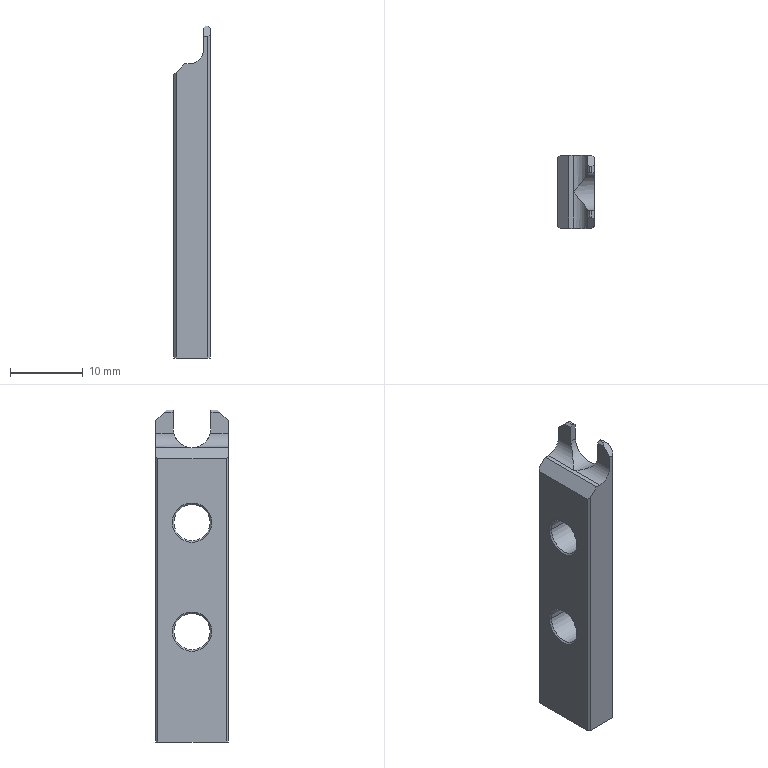Part | NX | 1 solid | 35 faces | box 5 x 10 x 45.7 mm | volume 1838 mm3 | plane 24 | cylinder 7 | cone 4 | commonest cylinder face diameters 5 x4 4 x2 5.2 x1
STEP:
#1=CARTESIAN_POINT('',(2162.7,155.748,-162.7));
#2=VERTEX_POINT('',#1);
#3=CARTESIAN_POINT('',(2163.,156.048,-162.7));
#4=VERTEX_POINT('',#3);
#5=CARTESIAN_POINT('',(2006.952,0.,-162.7));
#6=DIRECTION('',(0.7071,0.7071,0.));
#7=VECTOR('',#6,1000.);
#8=LINE('',#5,#7);
#9=EDGE_CURVE('',#2,#4,#8,.T.);
#10=ORIENTED_EDGE('',*,*,#9,.F.);
#11=CARTESIAN_POINT('',(2158.3,155.748,-162.7));
#12=VERTEX_POINT('',#11);
#13=CARTESIAN_POINT('',(0.,155.748,-162.7));
#14=DIRECTION('',(-1.,0.,0.));
#15=VECTOR('',#14,1000.);
#16=LINE('',#13,#15);
#17=EDGE_CURVE('',#2,#12,#16,.T.);
#18=ORIENTED_EDGE('',*,*,#17,.T.);
#19=CARTESIAN_POINT('',(2158.,156.048,-162.7));
#20=VERTEX_POINT('',#19);
#21=CARTESIAN_POINT('',(2314.048,0.,-162.7));
#22=DIRECTION('',(0.7071,-0.7071,0.));
#23=VECTOR('',#22,1000.);
#24=LINE('',#21,#23);
#25=EDGE_CURVE('',#20,#12,#24,.T.);
#26=ORIENTED_EDGE('',*,*,#25,.F.);
#27=CARTESIAN_POINT('',(2158.,165.448,-162.7));
#28=VERTEX_POINT('',#27);
#29=CARTESIAN_POINT('',(2158.,0.,-162.7));
#30=DIRECTION('',(0.,1.,0.));
#31=VECTOR('',#30,1000.);
#32=LINE('',#29,#31);
#33=EDGE_CURVE('',#20,#28,#32,.T.);
#34=ORIENTED_EDGE('',*,*,#33,.T.);
#35=CARTESIAN_POINT('',(2158.3,165.748,-162.7));
#36=VERTEX_POINT('',#35);
#37=CARTESIAN_POINT('',(1992.552,0.,-162.7));
#38=DIRECTION('',(-0.7071,-0.7071,0.));
#39=VECTOR('',#38,1000.);
#40=LINE('',#37,#39);
#41=EDGE_CURVE('',#36,#28,#40,.T.);
#42=ORIENTED_EDGE('',*,*,#41,.F.);
#43=CARTESIAN_POINT('',(2162.7,165.748,-162.7));
#44=VERTEX_POINT('',#43);
#45=CARTESIAN_POINT('',(0.,165.748,-162.7));
#46=DIRECTION('',(1.,0.,0.));
#47=VECTOR('',#46,1000.);
#48=LINE('',#45,#47);
#49=EDGE_CURVE('',#36,#44,#48,.T.);
#50=ORIENTED_EDGE('',*,*,#49,.T.);
#51=CARTESIAN_POINT('',(2163.,165.448,-162.7));
#52=VERTEX_POINT('',#51);
#53=CARTESIAN_POINT('',(2328.448,0.,-162.7));
#54=DIRECTION('',(0.7071,-0.7071,0.));
#55=VECTOR('',#54,1000.);
#56=LINE('',#53,#55);
#57=EDGE_CURVE('',#44,#52,#56,.T.);
#58=ORIENTED_EDGE('',*,*,#57,.T.);
#59=CARTESIAN_POINT('',(2163.,0.,-162.7));
#60=DIRECTION('',(0.,-1.,0.));
#61=VECTOR('',#60,1000.);
#62=LINE('',#59,#61);
#63=EDGE_CURVE('',#52,#4,#62,.T.);
#64=ORIENTED_EDGE('',*,*,#63,.T.);
#65=EDGE_LOOP('',(#10,#18,#26,#34,#42,#50,#58,#64));
#66=FACE_BOUND('',#65,.T.);
#67=CARTESIAN_POINT('',(2165.941,163.53,-162.7));
#68=DIRECTION('',(0.,0.,-1.));
#69=DIRECTION('',(0.,-1.,0.));
#70=AXIS2_PLACEMENT_3D('',#67,#68,#69);
#71=PLANE('',#70);
#72=ADVANCED_FACE('',(#66),#71,.T.);
#73=CARTESIAN_POINT('',(2162.7,155.748,-118.5));
#74=VERTEX_POINT('',#73);
#75=CARTESIAN_POINT('',(2162.7,155.748,0.));
#76=DIRECTION('',(0.,0.,1.));
#77=VECTOR('',#76,1000.);
#78=LINE('',#75,#77);
#79=EDGE_CURVE('',#2,#74,#78,.T.);
#80=ORIENTED_EDGE('',*,*,#79,.T.);
#81=CARTESIAN_POINT('',(2162.1,155.748,-118.5));
#82=VERTEX_POINT('',#81);
#83=CARTESIAN_POINT('',(2162.55,155.748,-118.5));
#84=DIRECTION('',(1.,0.,0.));
#85=VECTOR('',#84,1000.);
#86=LINE('',#83,#85);
#87=EDGE_CURVE('',#82,#74,#86,.T.);
#88=ORIENTED_EDGE('',*,*,#87,.F.);
#89=CARTESIAN_POINT('',(2162.1,155.748,-120.2));
#90=VERTEX_POINT('',#89);
#91=CARTESIAN_POINT('',(2162.1,155.748,-172.));
#92=DIRECTION('',(0.,0.,1.));
#93=VECTOR('',#92,1000.);
#94=LINE('',#91,#93);
#95=EDGE_CURVE('',#90,#82,#94,.T.);
#96=ORIENTED_EDGE('',*,*,#95,.F.);
#97=CARTESIAN_POINT('',(2160.1,155.748,-122.2));
#98=VERTEX_POINT('',#97);
#99=CARTESIAN_POINT('',(2160.1,155.748,-120.2));
#100=DIRECTION('',(0.,1.,0.));
#101=DIRECTION('',(-1.,0.,0.));
#102=AXIS2_PLACEMENT_3D('',#99,#100,#101);
#103=CIRCLE('',#102,2.);
#104=EDGE_CURVE('',#90,#98,#103,.T.);
#105=ORIENTED_EDGE('',*,*,#104,.T.);
#106=CARTESIAN_POINT('',(2159.5,155.748,-122.2));
#107=VERTEX_POINT('',#106);
#108=CARTESIAN_POINT('',(2165.941,155.748,-122.2));
#109=DIRECTION('',(1.,0.,0.));
#110=VECTOR('',#109,1000.);
#111=LINE('',#108,#110);
#112=EDGE_CURVE('',#107,#98,#111,.T.);
#113=ORIENTED_EDGE('',*,*,#112,.F.);
#114=CARTESIAN_POINT('',(2158.3,155.748,-123.4));
#115=VERTEX_POINT('',#114);
#116=CARTESIAN_POINT('',(2109.7,155.748,-172.));
#117=DIRECTION('',(-0.7071,0.,-0.7071));
#118=VECTOR('',#117,1000.);
#119=LINE('',#116,#118);
#120=EDGE_CURVE('',#107,#115,#119,.T.);
#121=ORIENTED_EDGE('',*,*,#120,.T.);
#122=CARTESIAN_POINT('',(2158.3,155.748,0.));
#123=DIRECTION('',(0.,0.,1.));
#124=VECTOR('',#123,1000.);
#125=LINE('',#122,#124);
#126=EDGE_CURVE('',#12,#115,#125,.T.);
#127=ORIENTED_EDGE('',*,*,#126,.F.);
#128=ORIENTED_EDGE('',*,*,#17,.F.);
#129=EDGE_LOOP('',(#80,#88,#96,#105,#113,#121,#127,#128));
#130=FACE_BOUND('',#129,.T.);
#131=CARTESIAN_POINT('',(2163.,155.748,-172.));
#132=DIRECTION('',(0.,-1.,0.));
#133=DIRECTION('',(0.,0.,-1.));
#134=AXIS2_PLACEMENT_3D('',#131,#132,#133);
#135=PLANE('',#134);
#136=ADVANCED_FACE('',(#130),#135,.T.);
#137=CARTESIAN_POINT('',(2163.,165.448,-118.2));
#138=VERTEX_POINT('',#137);
#139=CARTESIAN_POINT('',(2163.,165.448,0.));
#140=DIRECTION('',(0.,0.,1.));
#141=VECTOR('',#140,1000.);
#142=LINE('',#139,#141);
#143=EDGE_CURVE('',#52,#138,#142,.T.);
#144=ORIENTED_EDGE('',*,*,#143,.T.);
#145=CARTESIAN_POINT('',(2163.,164.548,-117.3));
#146=VERTEX_POINT('',#145);
#147=CARTESIAN_POINT('',(2163.,47.248,0.));
#148=DIRECTION('',(0.,-0.7071,0.7071));
#149=VECTOR('',#148,1000.);
#150=LINE('',#147,#149);
#151=EDGE_CURVE('',#138,#146,#150,.T.);
#152=ORIENTED_EDGE('',*,*,#151,.T.);
#153=CARTESIAN_POINT('',(2163.,163.348,-117.3));
#154=VERTEX_POINT('',#153);
#155=CARTESIAN_POINT('',(2163.,0.,-117.3));
#156=DIRECTION('',(0.,1.,0.));
#157=VECTOR('',#156,1000.);
#158=LINE('',#155,#157);
#159=EDGE_CURVE('',#154,#146,#158,.T.);
#160=ORIENTED_EDGE('',*,*,#159,.F.);
#161=CARTESIAN_POINT('',(2163.,163.348,-119.6));
#162=VERTEX_POINT('',#161);
#163=CARTESIAN_POINT('',(2163.,163.348,0.));
#164=DIRECTION('',(0.,0.,1.));
#165=VECTOR('',#164,1000.);
#166=LINE('',#163,#165);
#167=EDGE_CURVE('',#162,#154,#166,.T.);
#168=ORIENTED_EDGE('',*,*,#167,.F.);
#169=CARTESIAN_POINT('',(2163.,158.148,-119.6));
#170=VERTEX_POINT('',#169);
#171=CARTESIAN_POINT('',(2163.,160.748,-119.6));
#172=DIRECTION('',(1.,0.,0.));
#173=DIRECTION('',(0.,1.,0.));
#174=AXIS2_PLACEMENT_3D('',#171,#172,#173);
#175=CIRCLE('',#174,2.6);
#176=EDGE_CURVE('',#170,#162,#175,.T.);
#177=ORIENTED_EDGE('',*,*,#176,.F.);
#178=CARTESIAN_POINT('',(2163.,158.148,-117.3));
#179=VERTEX_POINT('',#178);
#180=CARTESIAN_POINT('',(2163.,158.148,0.));
#181=DIRECTION('',(0.,0.,-1.));
#182=VECTOR('',#181,1000.);
#183=LINE('',#180,#182);
#184=EDGE_CURVE('',#179,#170,#183,.T.);
#185=ORIENTED_EDGE('',*,*,#184,.F.);
#186=CARTESIAN_POINT('',(2163.,156.948,-117.3));
#187=VERTEX_POINT('',#186);
#188=CARTESIAN_POINT('',(2163.,156.948,-117.3));
#189=DIRECTION('',(0.,1.,0.));
#190=VECTOR('',#189,1000.);
#191=LINE('',#188,#190);
#192=EDGE_CURVE('',#187,#179,#191,.T.);
#193=ORIENTED_EDGE('',*,*,#192,.F.);
#194=CARTESIAN_POINT('',(2163.,156.048,-118.2));
#195=VERTEX_POINT('',#194);
#196=CARTESIAN_POINT('',(2163.,274.248,0.));
#197=DIRECTION('',(0.,-0.7071,-0.7071));
#198=VECTOR('',#197,1000.);
#199=LINE('',#196,#198);
#200=EDGE_CURVE('',#187,#195,#199,.T.);
#201=ORIENTED_EDGE('',*,*,#200,.T.);
#202=CARTESIAN_POINT('',(2163.,156.048,0.));
#203=DIRECTION('',(0.,0.,1.));
#204=VECTOR('',#203,1000.);
#205=LINE('',#202,#204);
#206=EDGE_CURVE('',#4,#195,#205,.T.);
#207=ORIENTED_EDGE('',*,*,#206,.F.);
#208=ORIENTED_EDGE('',*,*,#63,.F.);
#209=EDGE_LOOP('',(#144,#152,#160,#168,#177,#185,#193,#201,#207,#208));
#210=FACE_BOUND('',#209,.T.);
#211=CARTESIAN_POINT('',(2163.,158.248,-147.5));
#212=VERTEX_POINT('',#211);
#213=CARTESIAN_POINT('',(2163.,163.248,-147.5));
#214=VERTEX_POINT('',#213);
#215=CARTESIAN_POINT('',(2163.,160.748,-147.5));
#216=DIRECTION('',(-1.,0.,0.));
#217=DIRECTION('',(0.,-1.,0.));
#218=AXIS2_PLACEMENT_3D('',#215,#216,#217);
#219=CIRCLE('',#218,2.5);
#220=EDGE_CURVE('',#212,#214,#219,.T.);
#221=ORIENTED_EDGE('',*,*,#220,.T.);
#222=CARTESIAN_POINT('',(2163.,160.748,-147.5));
#223=DIRECTION('',(-1.,0.,0.));
#224=DIRECTION('',(0.,-1.,0.));
#225=AXIS2_PLACEMENT_3D('',#222,#223,#224);
#226=CIRCLE('',#225,2.5);
#227=EDGE_CURVE('',#214,#212,#226,.T.);
#228=ORIENTED_EDGE('',*,*,#227,.T.);
#229=EDGE_LOOP('',(#221,#228));
#230=FACE_BOUND('',#229,.T.);
#231=CARTESIAN_POINT('',(2163.,158.248,-132.5));
#232=VERTEX_POINT('',#231);
#233=CARTESIAN_POINT('',(2163.,163.248,-132.5));
#234=VERTEX_POINT('',#233);
#235=CARTESIAN_POINT('',(2163.,160.748,-132.5));
#236=DIRECTION('',(-1.,0.,0.));
#237=DIRECTION('',(0.,-1.,0.));
#238=AXIS2_PLACEMENT_3D('',#235,#236,#237);
#239=CIRCLE('',#238,2.5);
#240=EDGE_CURVE('',#232,#234,#239,.T.);
#241=ORIENTED_EDGE('',*,*,#240,.T.);
#242=CARTESIAN_POINT('',(2163.,160.748,-132.5));
#243=DIRECTION('',(-1.,0.,0.));
#244=DIRECTION('',(0.,-1.,0.));
#245=AXIS2_PLACEMENT_3D('',#242,#243,#244);
#246=CIRCLE('',#245,2.5);
#247=EDGE_CURVE('',#234,#232,#246,.T.);
#248=ORIENTED_EDGE('',*,*,#247,.T.);
#249=EDGE_LOOP('',(#241,#248));
#250=FACE_BOUND('',#249,.T.);
#251=CARTESIAN_POINT('',(2163.,165.748,-172.));
#252=DIRECTION('',(1.,0.,0.));
#253=DIRECTION('',(0.,1.,0.));
#254=AXIS2_PLACEMENT_3D('',#251,#252,#253);
#255=PLANE('',#254);
#256=ADVANCED_FACE('',(#210,#230,#250),#255,.T.);
#257=CARTESIAN_POINT('',(2158.3,165.748,-123.4));
#258=VERTEX_POINT('',#257);
#259=CARTESIAN_POINT('',(2158.3,165.748,-155.));
#260=DIRECTION('',(0.,0.,-1.));
#261=VECTOR('',#260,1000.);
#262=LINE('',#259,#261);
#263=EDGE_CURVE('',#258,#36,#262,.T.);
#264=ORIENTED_EDGE('',*,*,#263,.F.);
#265=CARTESIAN_POINT('',(2159.5,165.748,-122.2));
#266=VERTEX_POINT('',#265);
#267=CARTESIAN_POINT('',(2109.7,165.748,-172.));
#268=DIRECTION('',(0.7071,0.,0.7071));
#269=VECTOR('',#268,1000.);
#270=LINE('',#267,#269);
#271=EDGE_CURVE('',#258,#266,#270,.T.);
#272=ORIENTED_EDGE('',*,*,#271,.T.);
#273=CARTESIAN_POINT('',(2160.1,165.748,-122.2));
#274=VERTEX_POINT('',#273);
#275=CARTESIAN_POINT('',(2165.941,165.748,-122.2));
#276=DIRECTION('',(-1.,0.,0.));
#277=VECTOR('',#276,1000.);
#278=LINE('',#275,#277);
#279=EDGE_CURVE('',#274,#266,#278,.T.);
#280=ORIENTED_EDGE('',*,*,#279,.F.);
#281=CARTESIAN_POINT('',(2162.1,165.748,-120.2));
#282=VERTEX_POINT('',#281);
#283=CARTESIAN_POINT('',(2160.1,165.748,-120.2));
#284=DIRECTION('',(0.,1.,0.));
#285=DIRECTION('',(-1.,0.,0.));
#286=AXIS2_PLACEMENT_3D('',#283,#284,#285);
#287=CIRCLE('',#286,2.);
#288=EDGE_CURVE('',#282,#274,#287,.T.);
#289=ORIENTED_EDGE('',*,*,#288,.F.);
#290=CARTESIAN_POINT('',(2162.1,165.748,-118.5));
#291=VERTEX_POINT('',#290);
#292=CARTESIAN_POINT('',(2162.1,165.748,0.));
#293=DIRECTION('',(0.,0.,-1.));
#294=VECTOR('',#293,1000.);
#295=LINE('',#292,#294);
#296=EDGE_CURVE('',#291,#282,#295,.T.);
#297=ORIENTED_EDGE('',*,*,#296,.F.);
#298=CARTESIAN_POINT('',(2162.7,165.748,-118.5));
#299=VERTEX_POINT('',#298);
#300=CARTESIAN_POINT('',(2162.55,165.748,-118.5));
#301=DIRECTION('',(-1.,0.,0.));
#302=VECTOR('',#301,1000.);
#303=LINE('',#300,#302);
#304=EDGE_CURVE('',#299,#291,#303,.T.);
#305=ORIENTED_EDGE('',*,*,#304,.F.);
#306=CARTESIAN_POINT('',(2162.7,165.748,-155.));
#307=DIRECTION('',(0.,0.,-1.));
#308=VECTOR('',#307,1000.);
#309=LINE('',#306,#308);
#310=EDGE_CURVE('',#299,#44,#309,.T.);
#311=ORIENTED_EDGE('',*,*,#310,.T.);
#312=ORIENTED_EDGE('',*,*,#49,.F.);
#313=EDGE_LOOP('',(#264,#272,#280,#289,#297,#305,#311,#312));
#314=FACE_BOUND('',#313,.T.);
#315=CARTESIAN_POINT('',(2158.,165.748,-172.));
#316=DIRECTION('',(0.,1.,0.));
#317=DIRECTION('',(1.,0.,0.));
#318=AXIS2_PLACEMENT_3D('',#315,#316,#317);
#319=PLANE('',#318);
#320=ADVANCED_FACE('',(#314),#319,.T.);
#321=CARTESIAN_POINT('',(2158.,156.048,-123.7));
#322=VERTEX_POINT('',#321);
#323=CARTESIAN_POINT('',(2158.,156.048,-155.));
#324=DIRECTION('',(0.,0.,-1.));
#325=VECTOR('',#324,1000.);
#326=LINE('',#323,#325);
#327=EDGE_CURVE('',#322,#20,#326,.T.);
#328=ORIENTED_EDGE('',*,*,#327,.F.);
#329=CARTESIAN_POINT('',(2158.,165.448,-123.7));
#330=VERTEX_POINT('',#329);
#331=CARTESIAN_POINT('',(2158.,160.748,-123.7));
#332=DIRECTION('',(0.,-1.,0.));
#333=VECTOR('',#332,1000.);
#334=LINE('',#331,#333);
#335=EDGE_CURVE('',#330,#322,#334,.T.);
#336=ORIENTED_EDGE('',*,*,#335,.F.);
#337=CARTESIAN_POINT('',(2158.,165.448,0.));
#338=DIRECTION('',(0.,0.,1.));
#339=VECTOR('',#338,1000.);
#340=LINE('',#337,#339);
#341=EDGE_CURVE('',#28,#330,#340,.T.);
#342=ORIENTED_EDGE('',*,*,#341,.F.);
#343=ORIENTED_EDGE('',*,*,#33,.F.);
#344=EDGE_LOOP('',(#328,#336,#342,#343));
#345=FACE_BOUND('',#344,.T.);
#346=CARTESIAN_POINT('',(2158.,158.048,-147.5));
#347=VERTEX_POINT('',#346);
#348=CARTESIAN_POINT('',(2158.,163.448,-147.5));
#349=VERTEX_POINT('',#348);
#350=CARTESIAN_POINT('',(2158.,160.748,-147.5));
#351=DIRECTION('',(-1.,0.,0.));
#352=DIRECTION('',(0.,-1.,0.));
#353=AXIS2_PLACEMENT_3D('',#350,#351,#352);
#354=CIRCLE('',#353,2.7);
#355=EDGE_CURVE('',#347,#349,#354,.T.);
#356=ORIENTED_EDGE('',*,*,#355,.F.);
#357=CARTESIAN_POINT('',(2158.,160.748,-147.5));
#358=DIRECTION('',(-1.,0.,0.));
#359=DIRECTION('',(0.,-1.,0.));
#360=AXIS2_PLACEMENT_3D('',#357,#358,#359);
#361=CIRCLE('',#360,2.7);
#362=EDGE_CURVE('',#349,#347,#361,.T.);
#363=ORIENTED_EDGE('',*,*,#362,.F.);
#364=EDGE_LOOP('',(#356,#363));
#365=FACE_BOUND('',#364,.T.);
#366=CARTESIAN_POINT('',(2158.,163.448,-132.5));
#367=VERTEX_POINT('',#366);
#368=CARTESIAN_POINT('',(2158.,158.048,-132.5));
#369=VERTEX_POINT('',#368);
#370=CARTESIAN_POINT('',(2158.,160.748,-132.5));
#371=DIRECTION('',(-1.,0.,0.));
#372=DIRECTION('',(0.,-1.,0.));
#373=AXIS2_PLACEMENT_3D('',#370,#371,#372);
#374=CIRCLE('',#373,2.7);
#375=EDGE_CURVE('',#367,#369,#374,.T.);
#376=ORIENTED_EDGE('',*,*,#375,.F.);
#377=CARTESIAN_POINT('',(2158.,160.748,-132.5));
#378=DIRECTION('',(-1.,0.,0.));
#379=DIRECTION('',(0.,-1.,0.));
#380=AXIS2_PLACEMENT_3D('',#377,#378,#379);
#381=CIRCLE('',#380,2.7);
#382=EDGE_CURVE('',#369,#367,#381,.T.);
#383=ORIENTED_EDGE('',*,*,#382,.F.);
#384=EDGE_LOOP('',(#376,#383));
#385=FACE_BOUND('',#384,.T.);
#386=CARTESIAN_POINT('',(2158.,155.748,-172.));
#387=DIRECTION('',(-1.,0.,0.));
#388=DIRECTION('',(0.,0.,1.));
#389=AXIS2_PLACEMENT_3D('',#386,#387,#388);
#390=PLANE('',#389);
#391=ADVANCED_FACE('',(#345,#365,#385),#390,.T.);
#392=ORIENTED_EDGE('',*,*,#167,.T.);
#393=CARTESIAN_POINT('',(2162.7,163.348,-117.));
#394=VERTEX_POINT('',#393);
#395=CARTESIAN_POINT('',(0.,163.348,2045.7));
#396=DIRECTION('',(-0.7071,0.,0.7071));
#397=VECTOR('',#396,1000.);
#398=LINE('',#395,#397);
#399=EDGE_CURVE('',#154,#394,#398,.T.);
#400=ORIENTED_EDGE('',*,*,#399,.T.);
#401=CARTESIAN_POINT('',(2162.4,163.348,-117.));
#402=VERTEX_POINT('',#401);
#403=CARTESIAN_POINT('',(2162.1,163.348,-117.));
#404=DIRECTION('',(1.,0.,0.));
#405=VECTOR('',#404,1000.);
#406=LINE('',#403,#405);
#407=EDGE_CURVE('',#402,#394,#406,.T.);
#408=ORIENTED_EDGE('',*,*,#407,.F.);
#409=CARTESIAN_POINT('',(2162.1,163.348,-117.3));
#410=VERTEX_POINT('',#409);
#411=CARTESIAN_POINT('',(0.,163.348,-2279.4));
#412=DIRECTION('',(0.7071,0.,0.7071));
#413=VECTOR('',#412,1000.);
#414=LINE('',#411,#413);
#415=EDGE_CURVE('',#410,#402,#414,.T.);
#416=ORIENTED_EDGE('',*,*,#415,.F.);
#417=CARTESIAN_POINT('',(2162.1,163.348,-119.6));
#418=VERTEX_POINT('',#417);
#419=CARTESIAN_POINT('',(2162.1,163.348,0.));
#420=DIRECTION('',(0.,0.,1.));
#421=VECTOR('',#420,1000.);
#422=LINE('',#419,#421);
#423=EDGE_CURVE('',#418,#410,#422,.T.);
#424=ORIENTED_EDGE('',*,*,#423,.F.);
#425=CARTESIAN_POINT('',(2157.5,163.348,-119.6));
#426=DIRECTION('',(1.,0.,0.));
#427=VECTOR('',#426,1000.);
#428=LINE('',#425,#427);
#429=EDGE_CURVE('',#418,#162,#428,.T.);
#430=ORIENTED_EDGE('',*,*,#429,.T.);
#431=EDGE_LOOP('',(#392,#400,#408,#416,#424,#430));
#432=FACE_BOUND('',#431,.T.);
#433=CARTESIAN_POINT('',(2157.5,163.348,-117.));
#434=DIRECTION('',(0.,1.,0.));
#435=DIRECTION('',(0.,0.,-1.));
#436=AXIS2_PLACEMENT_3D('',#433,#434,#435);
#437=PLANE('',#436);
#438=ADVANCED_FACE('',(#432),#437,.F.);
#439=ORIENTED_EDGE('',*,*,#296,.T.);
#440=CARTESIAN_POINT('',(2162.1,163.277,-120.2));
#441=VERTEX_POINT('',#440);
#442=CARTESIAN_POINT('',(2162.1,163.53,-120.2));
#443=DIRECTION('',(0.,1.,0.));
#444=VECTOR('',#443,1000.);
#445=LINE('',#442,#444);
#446=EDGE_CURVE('',#441,#282,#445,.T.);
#447=ORIENTED_EDGE('',*,*,#446,.F.);
#448=CARTESIAN_POINT('',(2162.1,160.748,-119.6));
#449=DIRECTION('',(1.,0.,0.));
#450=DIRECTION('',(0.,1.,0.));
#451=AXIS2_PLACEMENT_3D('',#448,#449,#450);
#452=CIRCLE('',#451,2.6);
#453=EDGE_CURVE('',#441,#418,#452,.T.);
#454=ORIENTED_EDGE('',*,*,#453,.T.);
#455=ORIENTED_EDGE('',*,*,#423,.T.);
#456=CARTESIAN_POINT('',(2162.1,164.548,-117.3));
#457=VERTEX_POINT('',#456);
#458=CARTESIAN_POINT('',(2162.1,0.,-117.3));
#459=DIRECTION('',(0.,1.,0.));
#460=VECTOR('',#459,1000.);
#461=LINE('',#458,#460);
#462=EDGE_CURVE('',#410,#457,#461,.T.);
#463=ORIENTED_EDGE('',*,*,#462,.T.);
#464=CARTESIAN_POINT('',(2162.1,47.248,0.));
#465=DIRECTION('',(0.,-0.7071,0.7071));
#466=VECTOR('',#465,1000.);
#467=LINE('',#464,#466);
#468=EDGE_CURVE('',#291,#457,#467,.T.);
#469=ORIENTED_EDGE('',*,*,#468,.F.);
#470=EDGE_LOOP('',(#439,#447,#454,#455,#463,#469));
#471=FACE_BOUND('',#470,.T.);
#472=CARTESIAN_POINT('',(2162.1,154.748,-124.2));
#473=DIRECTION('',(1.,0.,0.));
#474=DIRECTION('',(0.,1.,0.));
#475=AXIS2_PLACEMENT_3D('',#472,#473,#474);
#476=PLANE('',#475);
#477=ADVANCED_FACE('',(#471),#476,.F.);
#478=CARTESIAN_POINT('',(2162.1,158.148,-117.3));
#479=VERTEX_POINT('',#478);
#480=CARTESIAN_POINT('',(2162.1,158.148,-119.6));
#481=VERTEX_POINT('',#480);
#482=CARTESIAN_POINT('',(2162.1,158.148,0.));
#483=DIRECTION('',(0.,0.,-1.));
#484=VECTOR('',#483,1000.);
#485=LINE('',#482,#484);
#486=EDGE_CURVE('',#479,#481,#485,.T.);
#487=ORIENTED_EDGE('',*,*,#486,.T.);
#488=CARTESIAN_POINT('',(2162.1,158.218,-120.2));
#489=VERTEX_POINT('',#488);
#490=CARTESIAN_POINT('',(2162.1,160.748,-119.6));
#491=DIRECTION('',(1.,0.,0.));
#492=DIRECTION('',(0.,1.,0.));
#493=AXIS2_PLACEMENT_3D('',#490,#491,#492);
#494=CIRCLE('',#493,2.6);
#495=EDGE_CURVE('',#481,#489,#494,.T.);
#496=ORIENTED_EDGE('',*,*,#495,.T.);
#497=CARTESIAN_POINT('',(2162.1,163.53,-120.2));
#498=DIRECTION('',(0.,1.,0.));
#499=VECTOR('',#498,1000.);
#500=LINE('',#497,#499);
#501=EDGE_CURVE('',#90,#489,#500,.T.);
#502=ORIENTED_EDGE('',*,*,#501,.F.);
#503=ORIENTED_EDGE('',*,*,#95,.T.);
#504=CARTESIAN_POINT('',(2162.1,156.948,-117.3));
#505=VERTEX_POINT('',#504);
#506=CARTESIAN_POINT('',(2162.1,274.248,0.));
#507=DIRECTION('',(0.,-0.7071,-0.7071));
#508=VECTOR('',#507,1000.);
#509=LINE('',#506,#508);
#510=EDGE_CURVE('',#505,#82,#509,.T.);
#511=ORIENTED_EDGE('',*,*,#510,.F.);
#512=CARTESIAN_POINT('',(2162.1,156.948,-117.3));
#513=DIRECTION('',(0.,1.,0.));
#514=VECTOR('',#513,1000.);
#515=LINE('',#512,#514);
#516=EDGE_CURVE('',#505,#479,#515,.T.);
#517=ORIENTED_EDGE('',*,*,#516,.T.);
#518=EDGE_LOOP('',(#487,#496,#502,#503,#511,#517));
#519=FACE_BOUND('',#518,.T.);
#520=CARTESIAN_POINT('',(2162.1,154.748,-124.2));
#521=DIRECTION('',(1.,0.,0.));
#522=DIRECTION('',(0.,1.,0.));
#523=AXIS2_PLACEMENT_3D('',#520,#521,#522);
#524=PLANE('',#523);
#525=ADVANCED_FACE('',(#519),#524,.F.);
#526=CARTESIAN_POINT('',(2159.5,160.748,-122.2));
#527=DIRECTION('',(0.,-1.,0.));
#528=VECTOR('',#527,1000.);
#529=LINE('',#526,#528);
#530=EDGE_CURVE('',#266,#107,#529,.T.);
#531=ORIENTED_EDGE('',*,*,#530,.T.);
#532=ORIENTED_EDGE('',*,*,#112,.T.);
#533=CARTESIAN_POINT('',(2160.1,160.748,-122.2));
#534=VERTEX_POINT('',#533);
#535=CARTESIAN_POINT('',(2160.1,163.53,-122.2));
#536=DIRECTION('',(0.,1.,0.));
#537=VECTOR('',#536,1000.);
#538=LINE('',#535,#537);
#539=EDGE_CURVE('',#98,#534,#538,.T.);
#540=ORIENTED_EDGE('',*,*,#539,.T.);
#541=CARTESIAN_POINT('',(2160.1,163.53,-122.2));
#542=DIRECTION('',(0.,1.,0.));
#543=VECTOR('',#542,1000.);
#544=LINE('',#541,#543);
#545=EDGE_CURVE('',#534,#274,#544,.T.);
#546=ORIENTED_EDGE('',*,*,#545,.T.);
#547=ORIENTED_EDGE('',*,*,#279,.T.);
#548=EDGE_LOOP('',(#531,#532,#540,#546,#547));
#549=FACE_BOUND('',#548,.T.);
#550=CARTESIAN_POINT('',(2158.,154.748,-122.2));
#551=DIRECTION('',(0.,0.,-1.));
#552=DIRECTION('',(0.,-1.,0.));
#553=AXIS2_PLACEMENT_3D('',#550,#551,#552);
#554=PLANE('',#553);
#555=ADVANCED_FACE('',(#549),#554,.F.);
#556=ORIENTED_EDGE('',*,*,#446,.T.);
#557=ORIENTED_EDGE('',*,*,#288,.T.);
#558=ORIENTED_EDGE('',*,*,#545,.F.);
#559=CARTESIAN_POINT('',(2160.1,160.748,-122.2));
#560=CARTESIAN_POINT('',(2160.212,160.876,-122.2));
#561=CARTESIAN_POINT('',(2160.325,161.004,-122.191));
#562=CARTESIAN_POINT('',(2160.436,161.131,-122.172));
#563=CARTESIAN_POINT('',(2160.492,161.195,-122.162));
#564=CARTESIAN_POINT('',(2160.547,161.259,-122.15));
#565=CARTESIAN_POINT('',(2160.603,161.322,-122.136));
#566=CARTESIAN_POINT('',(2160.63,161.354,-122.129));
#567=CARTESIAN_POINT('',(2160.658,161.385,-122.121));
#568=CARTESIAN_POINT('',(2160.685,161.417,-122.112));
#569=CARTESIAN_POINT('',(2160.713,161.448,-122.104));
#570=CARTESIAN_POINT('',(2160.74,161.48,-122.095));
#571=CARTESIAN_POINT('',(2160.767,161.511,-122.085));
#572=CARTESIAN_POINT('',(2160.822,161.574,-122.066));
#573=CARTESIAN_POINT('',(2160.876,161.636,-122.044));
#574=CARTESIAN_POINT('',(2160.929,161.698,-122.02));
#575=CARTESIAN_POINT('',(2160.982,161.76,-121.996));
#576=CARTESIAN_POINT('',(2161.035,161.821,-121.969));
#577=CARTESIAN_POINT('',(2161.087,161.882,-121.939));
#578=CARTESIAN_POINT('',(2161.113,161.913,-121.925));
#579=CARTESIAN_POINT('',(2161.139,161.943,-121.909));
#580=CARTESIAN_POINT('',(2161.164,161.973,-121.893));
#581=CARTESIAN_POINT('',(2161.19,162.003,-121.877));
#582=CARTESIAN_POINT('',(2161.215,162.033,-121.86));
#583=CARTESIAN_POINT('',(2161.24,162.063,-121.843));
#584=CARTESIAN_POINT('',(2161.291,162.122,-121.808));
#585=CARTESIAN_POINT('',(2161.34,162.181,-121.771));
#586=CARTESIAN_POINT('',(2161.388,162.239,-121.73));
#587=CARTESIAN_POINT('',(2161.436,162.296,-121.69));
#588=CARTESIAN_POINT('',(2161.483,162.353,-121.646));
#589=CARTESIAN_POINT('',(2161.528,162.409,-121.6));
#590=CARTESIAN_POINT('',(2161.551,162.436,-121.577));
#591=CARTESIAN_POINT('',(2161.573,162.464,-121.553));
#592=CARTESIAN_POINT('',(2161.595,162.491,-121.529));
#593=CARTESIAN_POINT('',(2161.617,162.519,-121.504));
#594=CARTESIAN_POINT('',(2161.638,162.546,-121.479));
#595=CARTESIAN_POINT('',(2161.659,162.572,-121.452));
#596=CARTESIAN_POINT('',(2161.68,162.599,-121.426));
#597=CARTESIAN_POINT('',(2161.701,162.625,-121.399));
#598=CARTESIAN_POINT('',(2161.721,162.651,-121.371));
#599=CARTESIAN_POINT('',(2161.741,162.677,-121.344));
#600=CARTESIAN_POINT('',(2161.761,162.702,-121.315));
#601=CARTESIAN_POINT('',(2161.78,162.727,-121.286));
#602=CARTESIAN_POINT('',(2161.799,162.752,-121.256));
#603=CARTESIAN_POINT('',(2161.817,162.777,-121.226));
#604=CARTESIAN_POINT('',(2161.835,162.801,-121.196));
#605=CARTESIAN_POINT('',(2161.852,162.824,-121.165));
#606=CARTESIAN_POINT('',(2161.869,162.848,-121.133));
#607=CARTESIAN_POINT('',(2161.886,162.871,-121.101));
#608=CARTESIAN_POINT('',(2161.902,162.893,-121.069));
#609=CARTESIAN_POINT('',(2161.917,162.916,-121.036));
#610=CARTESIAN_POINT('',(2161.932,162.937,-121.002));
#611=CARTESIAN_POINT('',(2161.947,162.959,-120.968));
#612=CARTESIAN_POINT('',(2161.961,162.98,-120.934));
#613=CARTESIAN_POINT('',(2161.974,163.,-120.899));
#614=CARTESIAN_POINT('',(2161.987,163.02,-120.864));
#615=CARTESIAN_POINT('',(2161.999,163.04,-120.828));
#616=CARTESIAN_POINT('',(2162.011,163.059,-120.791));
#617=CARTESIAN_POINT('',(2162.022,163.078,-120.754));
#618=CARTESIAN_POINT('',(2162.032,163.096,-120.717));
#619=CARTESIAN_POINT('',(2162.042,163.113,-120.679));
#620=CARTESIAN_POINT('',(2162.051,163.13,-120.641));
#621=CARTESIAN_POINT('',(2162.059,163.147,-120.603));
#622=CARTESIAN_POINT('',(2162.067,163.162,-120.564));
#623=CARTESIAN_POINT('',(2162.074,163.178,-120.525));
#624=CARTESIAN_POINT('',(2162.08,163.193,-120.485));
#625=CARTESIAN_POINT('',(2162.085,163.206,-120.445));
#626=CARTESIAN_POINT('',(2162.09,163.22,-120.405));
#627=CARTESIAN_POINT('',(2162.094,163.233,-120.364));
#628=CARTESIAN_POINT('',(2162.096,163.245,-120.324));
#629=CARTESIAN_POINT('',(2162.099,163.257,-120.283));
#630=CARTESIAN_POINT('',(2162.1,163.268,-120.241));
#631=CARTESIAN_POINT('',(2162.1,163.277,-120.2));
#632=B_SPLINE_CURVE_WITH_KNOTS('',3,(#559,#560,#561,#562,#563,#564,#565,#566,#567,#568,#569,#570,#571,#572,#573,#574,#575,#576,#577,#578,#579,#580,#581,#582,#583,#584,#585,#586,#587,#588,#589,#590,#591,#592,#593,#594,#595,#596,#597,#598,#599,#600,#601,#602,#603,#604,#605,#606,#607,#608,#609,#610,#611,#612,#613,#614,#615,#616,#617,#618,#619,#620,#621,#622,#623,#624,#625,#626,#627,#628,#629,#630,#631),.UNSPECIFIED.,.F.,.F.,(4,3,3,3,3,3,3,3,3,3,3,3,3,3,3,3,3,3,3,3,3,3,3,3,4),(0.,0.5111,0.7667,0.8945,1.022,1.278,1.534,1.662,1.79,2.046,2.301,2.43,2.558,2.687,2.816,2.944,3.073,3.201,3.329,3.457,3.585,3.713,3.841,3.969,4.097),.UNSPECIFIED.);
#633=EDGE_CURVE('',#534,#441,#632,.T.);
#634=ORIENTED_EDGE('',*,*,#633,.T.);
#635=EDGE_LOOP('',(#556,#557,#558,#634));
#636=FACE_BOUND('',#635,.T.);
#637=CARTESIAN_POINT('',(2160.1,163.53,-120.2));
#638=DIRECTION('',(0.,1.,0.));
#639=DIRECTION('',(-1.,0.,0.));
#640=AXIS2_PLACEMENT_3D('',#637,#638,#639);
#641=CYLINDRICAL_SURFACE('',#640,2.);
#642=ADVANCED_FACE('',(#636),#641,.F.);
#643=ORIENTED_EDGE('',*,*,#335,.T.);
#644=CARTESIAN_POINT('',(2109.7,204.348,-172.));
#645=DIRECTION('',(-0.5774,0.5774,-0.5774));
#646=VECTOR('',#645,1000.);
#647=LINE('',#644,#646);
#648=EDGE_CURVE('',#115,#322,#647,.T.);
#649=ORIENTED_EDGE('',*,*,#648,.F.);
#650=ORIENTED_EDGE('',*,*,#120,.F.);
#651=ORIENTED_EDGE('',*,*,#530,.F.);
#652=ORIENTED_EDGE('',*,*,#271,.F.);
#653=CARTESIAN_POINT('',(2156.083,163.53,-125.617));
#654=DIRECTION('',(-0.5774,-0.5774,-0.5774));
#655=VECTOR('',#654,1000.);
#656=LINE('',#653,#655);
#657=EDGE_CURVE('',#258,#330,#656,.T.);
#658=ORIENTED_EDGE('',*,*,#657,.T.);
#659=EDGE_LOOP('',(#643,#649,#650,#651,#652,#658));
#660=FACE_BOUND('',#659,.T.);
#661=CARTESIAN_POINT('',(2158.75,160.748,-122.95));
#662=DIRECTION('',(0.7071,0.,-0.7071));
#663=DIRECTION('',(0.,-1.,0.));
#664=AXIS2_PLACEMENT_3D('',#661,#662,#663);
#665=PLANE('',#664);
#666=ADVANCED_FACE('',(#660),#665,.F.);
#667=CARTESIAN_POINT('',(2158.2,163.248,-132.5));
#668=VERTEX_POINT('',#667);
#669=CARTESIAN_POINT('',(2158.2,158.248,-132.5));
#670=VERTEX_POINT('',#669);
#671=CARTESIAN_POINT('',(2158.2,160.748,-132.5));
#672=DIRECTION('',(-1.,0.,0.));
#673=DIRECTION('',(0.,-1.,0.));
#674=AXIS2_PLACEMENT_3D('',#671,#672,#673);
#675=CIRCLE('',#674,2.5);
#676=EDGE_CURVE('',#668,#670,#675,.T.);
#677=ORIENTED_EDGE('',*,*,#676,.T.);
#678=CARTESIAN_POINT('',(2158.,158.248,-132.5));
#679=DIRECTION('',(-1.,0.,0.));
#680=VECTOR('',#679,1000.);
#681=LINE('',#678,#680);
#682=EDGE_CURVE('',#670,#232,#681,.F.);
#683=ORIENTED_EDGE('',*,*,#682,.T.);
#684=ORIENTED_EDGE('',*,*,#247,.F.);
#685=CARTESIAN_POINT('',(2158.,163.248,-132.5));
#686=DIRECTION('',(-1.,0.,0.));
#687=VECTOR('',#686,1000.);
#688=LINE('',#685,#687);
#689=EDGE_CURVE('',#668,#234,#688,.F.);
#690=ORIENTED_EDGE('',*,*,#689,.F.);
#691=EDGE_LOOP('',(#677,#683,#684,#690));
#692=FACE_BOUND('',#691,.T.);
#693=CARTESIAN_POINT('',(2158.,160.748,-132.5));
#694=DIRECTION('',(-1.,0.,0.));
#695=DIRECTION('',(0.,-1.,0.));
#696=AXIS2_PLACEMENT_3D('',#693,#694,#695);
#697=CYLINDRICAL_SURFACE('',#696,2.5);
#698=ADVANCED_FACE('',(#692),#697,.F.);
#699=ORIENTED_EDGE('',*,*,#676,.F.);
#700=CARTESIAN_POINT('',(2158.2,163.248,-132.5));
#701=DIRECTION('',(-0.7071,0.7071,0.));
#702=VECTOR('',#701,1000.);
#703=LINE('',#700,#702);
#704=EDGE_CURVE('',#668,#367,#703,.T.);
#705=ORIENTED_EDGE('',*,*,#704,.T.);
#706=ORIENTED_EDGE('',*,*,#375,.T.);
#707=CARTESIAN_POINT('',(2158.2,158.248,-132.5));
#708=DIRECTION('',(-0.7071,-0.7071,0.));
#709=VECTOR('',#708,1000.);
#710=LINE('',#707,#709);
#711=EDGE_CURVE('',#670,#369,#710,.T.);
#712=ORIENTED_EDGE('',*,*,#711,.F.);
#713=EDGE_LOOP('',(#699,#705,#706,#712));
#714=FACE_BOUND('',#713,.T.);
#715=CARTESIAN_POINT('',(2158.2,160.748,-132.5));
#716=DIRECTION('',(-1.,0.,0.));
#717=DIRECTION('',(0.,1.,0.));
#718=AXIS2_PLACEMENT_3D('',#715,#716,#717);
#719=CONICAL_SURFACE('',#718,2.5,0.7854);
#720=ADVANCED_FACE('',(#714),#719,.F.);
#721=CARTESIAN_POINT('',(2158.2,163.248,-147.5));
#722=VERTEX_POINT('',#721);
#723=CARTESIAN_POINT('',(2158.2,158.248,-147.5));
#724=VERTEX_POINT('',#723);
#725=CARTESIAN_POINT('',(2158.2,160.748,-147.5));
#726=DIRECTION('',(-1.,0.,0.));
#727=DIRECTION('',(0.,-1.,0.));
#728=AXIS2_PLACEMENT_3D('',#725,#726,#727);
#729=CIRCLE('',#728,2.5);
#730=EDGE_CURVE('',#722,#724,#729,.T.);
#731=ORIENTED_EDGE('',*,*,#730,.T.);
#732=CARTESIAN_POINT('',(2158.,158.248,-147.5));
#733=DIRECTION('',(-1.,0.,0.));
#734=VECTOR('',#733,1000.);
#735=LINE('',#732,#734);
#736=EDGE_CURVE('',#724,#212,#735,.F.);
#737=ORIENTED_EDGE('',*,*,#736,.T.);
#738=ORIENTED_EDGE('',*,*,#227,.F.);
#739=CARTESIAN_POINT('',(2158.,163.248,-147.5));
#740=DIRECTION('',(-1.,0.,0.));
#741=VECTOR('',#740,1000.);
#742=LINE('',#739,#741);
#743=EDGE_CURVE('',#722,#214,#742,.F.);
#744=ORIENTED_EDGE('',*,*,#743,.F.);
#745=EDGE_LOOP('',(#731,#737,#738,#744));
#746=FACE_BOUND('',#745,.T.);
#747=CARTESIAN_POINT('',(2158.,160.748,-147.5));
#748=DIRECTION('',(-1.,0.,0.));
#749=DIRECTION('',(0.,-1.,0.));
#750=AXIS2_PLACEMENT_3D('',#747,#748,#749);
#751=CYLINDRICAL_SURFACE('',#750,2.5);
#752=ADVANCED_FACE('',(#746),#751,.F.);
#753=ORIENTED_EDGE('',*,*,#730,.F.);
#754=CARTESIAN_POINT('',(2158.2,163.248,-147.5));
#755=DIRECTION('',(-0.7071,0.7071,0.));
#756=VECTOR('',#755,1000.);
#757=LINE('',#754,#756);
#758=EDGE_CURVE('',#722,#349,#757,.T.);
#759=ORIENTED_EDGE('',*,*,#758,.T.);
#760=ORIENTED_EDGE('',*,*,#362,.T.);
#761=CARTESIAN_POINT('',(2158.2,158.248,-147.5));
#762=DIRECTION('',(-0.7071,-0.7071,0.));
#763=VECTOR('',#762,1000.);
#764=LINE('',#761,#763);
#765=EDGE_CURVE('',#724,#347,#764,.T.);
#766=ORIENTED_EDGE('',*,*,#765,.F.);
#767=EDGE_LOOP('',(#753,#759,#760,#766));
#768=FACE_BOUND('',#767,.T.);
#769=CARTESIAN_POINT('',(2158.2,160.748,-147.5));
#770=DIRECTION('',(-1.,0.,0.));
#771=DIRECTION('',(0.,1.,0.));
#772=AXIS2_PLACEMENT_3D('',#769,#770,#771);
#773=CONICAL_SURFACE('',#772,2.5,0.7854);
#774=ADVANCED_FACE('',(#768),#773,.F.);
#775=ORIENTED_EDGE('',*,*,#310,.F.);
#776=CARTESIAN_POINT('',(2281.2,47.248,0.));
#777=DIRECTION('',(0.5774,-0.5774,0.5774));
#778=VECTOR('',#777,1000.);
#779=LINE('',#776,#778);
#780=EDGE_CURVE('',#299,#138,#779,.T.);
#781=ORIENTED_EDGE('',*,*,#780,.T.);
#782=ORIENTED_EDGE('',*,*,#143,.F.);
#783=ORIENTED_EDGE('',*,*,#57,.F.);
#784=EDGE_LOOP('',(#775,#781,#782,#783));
#785=FACE_BOUND('',#784,.T.);
#786=CARTESIAN_POINT('',(2162.85,165.598,-136.15));
#787=DIRECTION('',(0.7071,0.7071,0.));
#788=DIRECTION('',(0.,0.,-1.));
#789=AXIS2_PLACEMENT_3D('',#786,#787,#788);
#790=PLANE('',#789);
#791=ADVANCED_FACE('',(#785),#790,.T.);
#792=ORIENTED_EDGE('',*,*,#341,.T.);
#793=ORIENTED_EDGE('',*,*,#657,.F.);
#794=ORIENTED_EDGE('',*,*,#263,.T.);
#795=ORIENTED_EDGE('',*,*,#41,.T.);
#796=EDGE_LOOP('',(#792,#793,#794,#795));
#797=FACE_BOUND('',#796,.T.);
#798=CARTESIAN_POINT('',(2158.15,165.598,-139.35));
#799=DIRECTION('',(-0.7071,0.7071,0.));
#800=DIRECTION('',(0.,0.,1.));
#801=AXIS2_PLACEMENT_3D('',#798,#799,#800);
#802=PLANE('',#801);
#803=ADVANCED_FACE('',(#797),#802,.T.);
#804=ORIENTED_EDGE('',*,*,#126,.T.);
#805=ORIENTED_EDGE('',*,*,#648,.T.);
#806=ORIENTED_EDGE('',*,*,#327,.T.);
#807=ORIENTED_EDGE('',*,*,#25,.T.);
#808=EDGE_LOOP('',(#804,#805,#806,#807));
#809=FACE_BOUND('',#808,.T.);
#810=CARTESIAN_POINT('',(2158.15,155.898,-139.35));
#811=DIRECTION('',(0.7071,0.7071,0.));
#812=DIRECTION('',(0.,0.,-1.));
#813=AXIS2_PLACEMENT_3D('',#810,#811,#812);
#814=PLANE('',#813);
#815=ADVANCED_FACE('',(#809),#814,.F.);
#816=ORIENTED_EDGE('',*,*,#206,.T.);
#817=CARTESIAN_POINT('',(2281.2,274.248,0.));
#818=DIRECTION('',(-0.5774,-0.5774,-0.5774));
#819=VECTOR('',#818,1000.);
#820=LINE('',#817,#819);
#821=EDGE_CURVE('',#195,#74,#820,.T.);
#822=ORIENTED_EDGE('',*,*,#821,.T.);
#823=ORIENTED_EDGE('',*,*,#79,.F.);
#824=ORIENTED_EDGE('',*,*,#9,.T.);
#825=EDGE_LOOP('',(#816,#822,#823,#824));
#826=FACE_BOUND('',#825,.T.);
#827=CARTESIAN_POINT('',(2162.85,155.898,-136.15));
#828=DIRECTION('',(0.7071,-0.7071,0.));
#829=DIRECTION('',(0.,0.,-1.));
#830=AXIS2_PLACEMENT_3D('',#827,#828,#829);
#831=PLANE('',#830);
#832=ADVANCED_FACE('',(#826),#831,.T.);
#833=CARTESIAN_POINT('',(2162.713,158.148,-117.013));
#834=VERTEX_POINT('',#833);
#835=CARTESIAN_POINT('',(2162.387,158.148,-117.013));
#836=VERTEX_POINT('',#835);
#837=CARTESIAN_POINT('',(0.,158.148,-117.013));
#838=DIRECTION('',(-1.,0.,0.));
#839=VECTOR('',#838,1000.);
#840=LINE('',#837,#839);
#841=EDGE_CURVE('',#834,#836,#840,.T.);
#842=ORIENTED_EDGE('',*,*,#841,.F.);
#843=CARTESIAN_POINT('',(0.,158.148,2045.7));
#844=DIRECTION('',(0.7071,0.,-0.7071));
#845=VECTOR('',#844,1000.);
#846=LINE('',#843,#845);
#847=EDGE_CURVE('',#834,#179,#846,.T.);
#848=ORIENTED_EDGE('',*,*,#847,.T.);
#849=ORIENTED_EDGE('',*,*,#184,.T.);
#850=CARTESIAN_POINT('',(2157.5,158.148,-119.6));
#851=DIRECTION('',(1.,0.,0.));
#852=VECTOR('',#851,1000.);
#853=LINE('',#850,#852);
#854=EDGE_CURVE('',#481,#170,#853,.T.);
#855=ORIENTED_EDGE('',*,*,#854,.F.);
#856=ORIENTED_EDGE('',*,*,#486,.F.);
#857=CARTESIAN_POINT('',(0.,158.148,-2279.4));
#858=DIRECTION('',(-0.7071,0.,-0.7071));
#859=VECTOR('',#858,1000.);
#860=LINE('',#857,#859);
#861=EDGE_CURVE('',#836,#479,#860,.T.);
#862=ORIENTED_EDGE('',*,*,#861,.F.);
#863=EDGE_LOOP('',(#842,#848,#849,#855,#856,#862));
#864=FACE_BOUND('',#863,.T.);
#865=CARTESIAN_POINT('',(2157.5,158.148,-119.6));
#866=DIRECTION('',(0.,-1.,0.));
#867=DIRECTION('',(-1.,0.,0.));
#868=AXIS2_PLACEMENT_3D('',#865,#866,#867);
#869=PLANE('',#868);
#870=ADVANCED_FACE('',(#864),#869,.F.);
#871=ORIENTED_EDGE('',*,*,#87,.T.);
#872=ORIENTED_EDGE('',*,*,#821,.F.);
#873=ORIENTED_EDGE('',*,*,#200,.F.);
#874=CARTESIAN_POINT('',(2162.7,157.248,-117.));
#875=VERTEX_POINT('',#874);
#876=CARTESIAN_POINT('',(0.,2319.948,2045.7));
#877=DIRECTION('',(0.5774,-0.5774,-0.5774));
#878=VECTOR('',#877,1000.);
#879=LINE('',#876,#878);
#880=EDGE_CURVE('',#875,#187,#879,.T.);
#881=ORIENTED_EDGE('',*,*,#880,.F.);
#882=CARTESIAN_POINT('',(2162.4,157.248,-117.));
#883=VERTEX_POINT('',#882);
#884=CARTESIAN_POINT('',(2162.55,157.248,-117.));
#885=DIRECTION('',(1.,0.,0.));
#886=VECTOR('',#885,1000.);
#887=LINE('',#884,#886);
#888=EDGE_CURVE('',#883,#875,#887,.T.);
#889=ORIENTED_EDGE('',*,*,#888,.F.);
#890=CARTESIAN_POINT('',(0.,-2005.152,-2279.4));
#891=DIRECTION('',(-0.5774,-0.5774,-0.5774));
#892=VECTOR('',#891,1000.);
#893=LINE('',#890,#892);
#894=EDGE_CURVE('',#883,#505,#893,.T.);
#895=ORIENTED_EDGE('',*,*,#894,.T.);
#896=ORIENTED_EDGE('',*,*,#510,.T.);
#897=EDGE_LOOP('',(#871,#872,#873,#881,#889,#895,#896));
#898=FACE_BOUND('',#897,.T.);
#899=CARTESIAN_POINT('',(2162.55,156.498,-117.75));
#900=DIRECTION('',(0.,0.7071,-0.7071));
#901=DIRECTION('',(-1.,0.,0.));
#902=AXIS2_PLACEMENT_3D('',#899,#900,#901);
#903=PLANE('',#902);
#904=ADVANCED_FACE('',(#898),#903,.F.);
#905=ORIENTED_EDGE('',*,*,#304,.T.);
#906=ORIENTED_EDGE('',*,*,#468,.T.);
#907=CARTESIAN_POINT('',(2162.4,164.248,-117.));
#908=VERTEX_POINT('',#907);
#909=CARTESIAN_POINT('',(0.,2326.648,-2279.4));
#910=DIRECTION('',(0.5774,-0.5774,0.5774));
#911=VECTOR('',#910,1000.);
#912=LINE('',#909,#911);
#913=EDGE_CURVE('',#457,#908,#912,.T.);
#914=ORIENTED_EDGE('',*,*,#913,.T.);
#915=CARTESIAN_POINT('',(2162.7,164.248,-117.));
#916=VERTEX_POINT('',#915);
#917=CARTESIAN_POINT('',(2162.55,164.248,-117.));
#918=DIRECTION('',(-1.,0.,0.));
#919=VECTOR('',#918,1000.);
#920=LINE('',#917,#919);
#921=EDGE_CURVE('',#916,#908,#920,.T.);
#922=ORIENTED_EDGE('',*,*,#921,.F.);
#923=CARTESIAN_POINT('',(0.,-1998.452,2045.7));
#924=DIRECTION('',(-0.5774,-0.5774,0.5774));
#925=VECTOR('',#924,1000.);
#926=LINE('',#923,#925);
#927=EDGE_CURVE('',#146,#916,#926,.T.);
#928=ORIENTED_EDGE('',*,*,#927,.F.);
#929=ORIENTED_EDGE('',*,*,#151,.F.);
#930=ORIENTED_EDGE('',*,*,#780,.F.);
#931=EDGE_LOOP('',(#905,#906,#914,#922,#928,#929,#930));
#932=FACE_BOUND('',#931,.T.);
#933=CARTESIAN_POINT('',(2162.55,164.998,-117.75));
#934=DIRECTION('',(0.,-0.7071,-0.7071));
#935=DIRECTION('',(0.,-0.7071,0.7071));
#936=AXIS2_PLACEMENT_3D('',#933,#934,#935);
#937=PLANE('',#936);
#938=ADVANCED_FACE('',(#932),#937,.F.);
#939=ORIENTED_EDGE('',*,*,#453,.F.);
#940=ORIENTED_EDGE('',*,*,#633,.F.);
#941=CARTESIAN_POINT('',(2162.1,158.218,-120.2));
#942=CARTESIAN_POINT('',(2162.1,158.228,-120.241));
#943=CARTESIAN_POINT('',(2162.099,158.239,-120.283));
#944=CARTESIAN_POINT('',(2162.096,158.25,-120.324));
#945=CARTESIAN_POINT('',(2162.094,158.262,-120.364));
#946=CARTESIAN_POINT('',(2162.09,158.275,-120.405));
#947=CARTESIAN_POINT('',(2162.085,158.289,-120.445));
#948=CARTESIAN_POINT('',(2162.08,158.303,-120.485));
#949=CARTESIAN_POINT('',(2162.074,158.317,-120.525));
#950=CARTESIAN_POINT('',(2162.067,158.333,-120.564));
#951=CARTESIAN_POINT('',(2162.059,158.348,-120.603));
#952=CARTESIAN_POINT('',(2162.051,158.365,-120.641));
#953=CARTESIAN_POINT('',(2162.042,158.382,-120.679));
#954=CARTESIAN_POINT('',(2162.032,158.4,-120.717));
#955=CARTESIAN_POINT('',(2162.022,158.418,-120.754));
#956=CARTESIAN_POINT('',(2162.011,158.437,-120.791));
#957=CARTESIAN_POINT('',(2161.999,158.455,-120.828));
#958=CARTESIAN_POINT('',(2161.987,158.475,-120.864));
#959=CARTESIAN_POINT('',(2161.974,158.495,-120.899));
#960=CARTESIAN_POINT('',(2161.961,158.516,-120.934));
#961=CARTESIAN_POINT('',(2161.947,158.537,-120.968));
#962=CARTESIAN_POINT('',(2161.932,158.558,-121.002));
#963=CARTESIAN_POINT('',(2161.917,158.58,-121.036));
#964=CARTESIAN_POINT('',(2161.902,158.602,-121.069));
#965=CARTESIAN_POINT('',(2161.886,158.625,-121.101));
#966=CARTESIAN_POINT('',(2161.869,158.647,-121.133));
#967=CARTESIAN_POINT('',(2161.852,158.671,-121.165));
#968=CARTESIAN_POINT('',(2161.835,158.695,-121.196));
#969=CARTESIAN_POINT('',(2161.817,158.719,-121.226));
#970=CARTESIAN_POINT('',(2161.799,158.743,-121.256));
#971=CARTESIAN_POINT('',(2161.78,158.768,-121.286));
#972=CARTESIAN_POINT('',(2161.761,158.793,-121.315));
#973=CARTESIAN_POINT('',(2161.741,158.819,-121.344));
#974=CARTESIAN_POINT('',(2161.721,158.844,-121.371));
#975=CARTESIAN_POINT('',(2161.701,158.87,-121.399));
#976=CARTESIAN_POINT('',(2161.68,158.897,-121.426));
#977=CARTESIAN_POINT('',(2161.659,158.923,-121.452));
#978=CARTESIAN_POINT('',(2161.638,158.95,-121.479));
#979=CARTESIAN_POINT('',(2161.617,158.977,-121.504));
#980=CARTESIAN_POINT('',(2161.595,159.004,-121.529));
#981=CARTESIAN_POINT('',(2161.573,159.031,-121.553));
#982=CARTESIAN_POINT('',(2161.551,159.059,-121.577));
#983=CARTESIAN_POINT('',(2161.528,159.087,-121.6));
#984=CARTESIAN_POINT('',(2161.483,159.142,-121.646));
#985=CARTESIAN_POINT('',(2161.436,159.199,-121.69));
#986=CARTESIAN_POINT('',(2161.388,159.257,-121.73));
#987=CARTESIAN_POINT('',(2161.34,159.315,-121.771));
#988=CARTESIAN_POINT('',(2161.291,159.373,-121.808));
#989=CARTESIAN_POINT('',(2161.24,159.433,-121.843));
#990=CARTESIAN_POINT('',(2161.215,159.462,-121.86));
#991=CARTESIAN_POINT('',(2161.19,159.492,-121.877));
#992=CARTESIAN_POINT('',(2161.164,159.522,-121.893));
#993=CARTESIAN_POINT('',(2161.139,159.552,-121.909));
#994=CARTESIAN_POINT('',(2161.113,159.583,-121.925));
#995=CARTESIAN_POINT('',(2161.087,159.613,-121.939));
#996=CARTESIAN_POINT('',(2161.035,159.674,-121.969));
#997=CARTESIAN_POINT('',(2160.982,159.735,-121.996));
#998=CARTESIAN_POINT('',(2160.929,159.797,-122.02));
#999=CARTESIAN_POINT('',(2160.876,159.859,-122.044));
#1000=CARTESIAN_POINT('',(2160.822,159.922,-122.066));
#1001=CARTESIAN_POINT('',(2160.767,159.984,-122.085));
#1002=CARTESIAN_POINT('',(2160.74,160.016,-122.095));
#1003=CARTESIAN_POINT('',(2160.713,160.047,-122.104));
#1004=CARTESIAN_POINT('',(2160.685,160.079,-122.112));
#1005=CARTESIAN_POINT('',(2160.658,160.11,-122.121));
#1006=CARTESIAN_POINT('',(2160.63,160.142,-122.129));
#1007=CARTESIAN_POINT('',(2160.603,160.173,-122.136));
#1008=CARTESIAN_POINT('',(2160.547,160.237,-122.15));
#1009=CARTESIAN_POINT('',(2160.492,160.3,-122.162));
#1010=CARTESIAN_POINT('',(2160.436,160.364,-122.172));
#1011=CARTESIAN_POINT('',(2160.325,160.491,-122.191));
#1012=CARTESIAN_POINT('',(2160.212,160.62,-122.2));
#1013=CARTESIAN_POINT('',(2160.1,160.748,-122.2));
#1014=B_SPLINE_CURVE_WITH_KNOTS('',3,(#941,#942,#943,#944,#945,#946,#947,#948,#949,#950,#951,#952,#953,#954,#955,#956,#957,#958,#959,#960,#961,#962,#963,#964,#965,#966,#967,#968,#969,#970,#971,#972,#973,#974,#975,#976,#977,#978,#979,#980,#981,#982,#983,#984,#985,#986,#987,#988,#989,#990,#991,#992,#993,#994,#995,#996,#997,#998,#999,#1000,#1001,#1002,#1003,#1004,#1005,#1006,#1007,#1008,#1009,#1010,#1011,#1012,#1013),.UNSPECIFIED.,.F.,.F.,(4,3,3,3,3,3,3,3,3,3,3,3,3,3,3,3,3,3,3,3,3,3,3,3,4),(0.,0.1279,0.2559,0.3839,0.5118,0.6399,0.7682,0.8961,1.024,1.152,1.281,1.41,1.538,1.667,1.795,2.051,2.307,2.435,2.563,2.818,3.074,3.202,3.33,3.586,4.097),.UNSPECIFIED.);
#1015=EDGE_CURVE('',#489,#534,#1014,.T.);
#1016=ORIENTED_EDGE('',*,*,#1015,.F.);
#1017=ORIENTED_EDGE('',*,*,#495,.F.);
#1018=ORIENTED_EDGE('',*,*,#854,.T.);
#1019=ORIENTED_EDGE('',*,*,#176,.T.);
#1020=ORIENTED_EDGE('',*,*,#429,.F.);
#1021=EDGE_LOOP('',(#939,#940,#1016,#1017,#1018,#1019,#1020));
#1022=FACE_BOUND('',#1021,.T.);
#1023=CARTESIAN_POINT('',(2157.5,160.748,-119.6));
#1024=DIRECTION('',(1.,0.,0.));
#1025=DIRECTION('',(0.,1.,0.));
#1026=AXIS2_PLACEMENT_3D('',#1023,#1024,#1025);
#1027=CYLINDRICAL_SURFACE('',#1026,2.6);
#1028=ADVANCED_FACE('',(#1022),#1027,.F.);
#1029=CARTESIAN_POINT('',(2162.4,0.,-117.));
#1030=DIRECTION('',(0.,1.,0.));
#1031=VECTOR('',#1030,1000.);
#1032=LINE('',#1029,#1031);
#1033=EDGE_CURVE('',#402,#908,#1032,.T.);
#1034=ORIENTED_EDGE('',*,*,#1033,.F.);
#1035=ORIENTED_EDGE('',*,*,#407,.T.);
#1036=CARTESIAN_POINT('',(2162.7,0.,-117.));
#1037=DIRECTION('',(0.,1.,0.));
#1038=VECTOR('',#1037,1000.);
#1039=LINE('',#1036,#1038);
#1040=EDGE_CURVE('',#394,#916,#1039,.T.);
#1041=ORIENTED_EDGE('',*,*,#1040,.T.);
#1042=ORIENTED_EDGE('',*,*,#921,.T.);
#1043=EDGE_LOOP('',(#1034,#1035,#1041,#1042));
#1044=FACE_BOUND('',#1043,.T.);
#1045=CARTESIAN_POINT('',(2165.941,163.53,-117.));
#1046=DIRECTION('',(0.,0.,-1.));
#1047=DIRECTION('',(0.,-1.,0.));
#1048=AXIS2_PLACEMENT_3D('',#1045,#1046,#1047);
#1049=PLANE('',#1048);
#1050=ADVANCED_FACE('',(#1044),#1049,.F.);
#1051=CARTESIAN_POINT('',(2162.4,158.148,-117.));
#1052=VERTEX_POINT('',#1051);
#1053=CARTESIAN_POINT('',(2162.4,156.948,-117.));
#1054=DIRECTION('',(0.,1.,0.));
#1055=VECTOR('',#1054,1000.);
#1056=LINE('',#1053,#1055);
#1057=EDGE_CURVE('',#883,#1052,#1056,.T.);
#1058=ORIENTED_EDGE('',*,*,#1057,.F.);
#1059=ORIENTED_EDGE('',*,*,#888,.T.);
#1060=CARTESIAN_POINT('',(2162.7,158.148,-117.));
#1061=VERTEX_POINT('',#1060);
#1062=CARTESIAN_POINT('',(2162.7,156.948,-117.));
#1063=DIRECTION('',(0.,1.,0.));
#1064=VECTOR('',#1063,1000.);
#1065=LINE('',#1062,#1064);
#1066=EDGE_CURVE('',#875,#1061,#1065,.T.);
#1067=ORIENTED_EDGE('',*,*,#1066,.T.);
#1068=CARTESIAN_POINT('',(2165.941,158.148,-117.));
#1069=DIRECTION('',(-1.,0.,0.));
#1070=VECTOR('',#1069,1000.);
#1071=LINE('',#1068,#1070);
#1072=EDGE_CURVE('',#1061,#1052,#1071,.T.);
#1073=ORIENTED_EDGE('',*,*,#1072,.T.);
#1074=EDGE_LOOP('',(#1058,#1059,#1067,#1073));
#1075=FACE_BOUND('',#1074,.T.);
#1076=CARTESIAN_POINT('',(2165.941,163.53,-117.));
#1077=DIRECTION('',(0.,0.,-1.));
#1078=DIRECTION('',(0.,-1.,0.));
#1079=AXIS2_PLACEMENT_3D('',#1076,#1077,#1078);
#1080=PLANE('',#1079);
#1081=ADVANCED_FACE('',(#1075),#1080,.F.);
#1082=ORIENTED_EDGE('',*,*,#1066,.F.);
#1083=ORIENTED_EDGE('',*,*,#880,.T.);
#1084=ORIENTED_EDGE('',*,*,#192,.T.);
#1085=ORIENTED_EDGE('',*,*,#847,.F.);
#1086=CARTESIAN_POINT('',(2165.941,158.18,-120.241));
#1087=DIRECTION('',(0.7071,0.007061,-0.7071));
#1088=VECTOR('',#1087,1000.);
#1089=LINE('',#1086,#1088);
#1090=EDGE_CURVE('',#1061,#834,#1089,.T.);
#1091=ORIENTED_EDGE('',*,*,#1090,.F.);
#1092=EDGE_LOOP('',(#1082,#1083,#1084,#1085,#1091));
#1093=FACE_BOUND('',#1092,.T.);
#1094=CARTESIAN_POINT('',(2162.85,156.948,-117.15));
#1095=DIRECTION('',(0.7071,0.,0.7071));
#1096=DIRECTION('',(0.,-1.,0.));
#1097=AXIS2_PLACEMENT_3D('',#1094,#1095,#1096);
#1098=PLANE('',#1097);
#1099=ADVANCED_FACE('',(#1093),#1098,.T.);
#1100=ORIENTED_EDGE('',*,*,#1040,.F.);
#1101=ORIENTED_EDGE('',*,*,#399,.F.);
#1102=ORIENTED_EDGE('',*,*,#159,.T.);
#1103=ORIENTED_EDGE('',*,*,#927,.T.);
#1104=EDGE_LOOP('',(#1100,#1101,#1102,#1103));
#1105=FACE_BOUND('',#1104,.T.);
#1106=CARTESIAN_POINT('',(2162.85,164.548,-117.15));
#1107=DIRECTION('',(0.7071,0.,0.7071));
#1108=DIRECTION('',(0.,-1.,0.));
#1109=AXIS2_PLACEMENT_3D('',#1106,#1107,#1108);
#1110=PLANE('',#1109);
#1111=ADVANCED_FACE('',(#1105),#1110,.T.);
#1112=ORIENTED_EDGE('',*,*,#1033,.T.);
#1113=ORIENTED_EDGE('',*,*,#913,.F.);
#1114=ORIENTED_EDGE('',*,*,#462,.F.);
#1115=ORIENTED_EDGE('',*,*,#415,.T.);
#1116=EDGE_LOOP('',(#1112,#1113,#1114,#1115));
#1117=FACE_BOUND('',#1116,.T.);
#1118=CARTESIAN_POINT('',(2162.25,164.548,-117.15));
#1119=DIRECTION('',(0.7071,0.,-0.7071));
#1120=DIRECTION('',(0.,-1.,0.));
#1121=AXIS2_PLACEMENT_3D('',#1118,#1119,#1120);
#1122=PLANE('',#1121);
#1123=ADVANCED_FACE('',(#1117),#1122,.F.);
#1124=ORIENTED_EDGE('',*,*,#1057,.T.);
#1125=CARTESIAN_POINT('',(2165.941,158.112,-113.459));
#1126=DIRECTION('',(-0.7071,0.007061,-0.7071));
#1127=VECTOR('',#1126,1000.);
#1128=LINE('',#1125,#1127);
#1129=EDGE_CURVE('',#1052,#836,#1128,.T.);
#1130=ORIENTED_EDGE('',*,*,#1129,.T.);
#1131=ORIENTED_EDGE('',*,*,#861,.T.);
#1132=ORIENTED_EDGE('',*,*,#516,.F.);
#1133=ORIENTED_EDGE('',*,*,#894,.F.);
#1134=EDGE_LOOP('',(#1124,#1130,#1131,#1132,#1133));
#1135=FACE_BOUND('',#1134,.T.);
#1136=CARTESIAN_POINT('',(2162.25,156.948,-117.15));
#1137=DIRECTION('',(0.7071,0.,-0.7071));
#1138=DIRECTION('',(0.,-1.,0.));
#1139=AXIS2_PLACEMENT_3D('',#1136,#1137,#1138);
#1140=PLANE('',#1139);
#1141=ADVANCED_FACE('',(#1135),#1140,.F.);
#1142=ORIENTED_EDGE('',*,*,#1015,.T.);
#1143=ORIENTED_EDGE('',*,*,#539,.F.);
#1144=ORIENTED_EDGE('',*,*,#104,.F.);
#1145=ORIENTED_EDGE('',*,*,#501,.T.);
#1146=EDGE_LOOP('',(#1142,#1143,#1144,#1145));
#1147=FACE_BOUND('',#1146,.T.);
#1148=CARTESIAN_POINT('',(2160.1,163.53,-120.2));
#1149=DIRECTION('',(0.,1.,0.));
#1150=DIRECTION('',(-1.,0.,0.));
#1151=AXIS2_PLACEMENT_3D('',#1148,#1149,#1150);
#1152=CYLINDRICAL_SURFACE('',#1151,2.);
#1153=ADVANCED_FACE('',(#1147),#1152,.F.);
#1154=ORIENTED_EDGE('',*,*,#841,.T.);
#1155=ORIENTED_EDGE('',*,*,#1129,.F.);
#1156=ORIENTED_EDGE('',*,*,#1072,.F.);
#1157=ORIENTED_EDGE('',*,*,#1090,.T.);
#1158=EDGE_LOOP('',(#1154,#1155,#1156,#1157));
#1159=FACE_BOUND('',#1158,.T.);
#1160=CARTESIAN_POINT('',(2157.5,158.148,-117.026));
#1161=DIRECTION('',(0.,-1.,-0.009985));
#1162=DIRECTION('',(0.,0.009985,-1.));
#1163=AXIS2_PLACEMENT_3D('',#1160,#1161,#1162);
#1164=PLANE('',#1163);
#1165=ADVANCED_FACE('',(#1159),#1164,.F.);
#1166=ORIENTED_EDGE('',*,*,#704,.F.);
#1167=CARTESIAN_POINT('',(2158.2,160.748,-132.5));
#1168=DIRECTION('',(-1.,0.,0.));
#1169=DIRECTION('',(0.,-1.,0.));
#1170=AXIS2_PLACEMENT_3D('',#1167,#1168,#1169);
#1171=CIRCLE('',#1170,2.5);
#1172=EDGE_CURVE('',#670,#668,#1171,.T.);
#1173=ORIENTED_EDGE('',*,*,#1172,.F.);
#1174=ORIENTED_EDGE('',*,*,#711,.T.);
#1175=ORIENTED_EDGE('',*,*,#382,.T.);
#1176=EDGE_LOOP('',(#1166,#1173,#1174,#1175));
#1177=FACE_BOUND('',#1176,.T.);
#1178=CARTESIAN_POINT('',(2158.2,160.748,-132.5));
#1179=DIRECTION('',(-1.,0.,0.));
#1180=DIRECTION('',(0.,1.,0.));
#1181=AXIS2_PLACEMENT_3D('',#1178,#1179,#1180);
#1182=CONICAL_SURFACE('',#1181,2.5,0.7854);
#1183=ADVANCED_FACE('',(#1177),#1182,.F.);
#1184=ORIENTED_EDGE('',*,*,#240,.F.);
#1185=ORIENTED_EDGE('',*,*,#682,.F.);
#1186=ORIENTED_EDGE('',*,*,#1172,.T.);
#1187=ORIENTED_EDGE('',*,*,#689,.T.);
#1188=EDGE_LOOP('',(#1184,#1185,#1186,#1187));
#1189=FACE_BOUND('',#1188,.T.);
#1190=CARTESIAN_POINT('',(2158.,160.748,-132.5));
#1191=DIRECTION('',(-1.,0.,0.));
#1192=DIRECTION('',(0.,-1.,0.));
#1193=AXIS2_PLACEMENT_3D('',#1190,#1191,#1192);
#1194=CYLINDRICAL_SURFACE('',#1193,2.5);
#1195=ADVANCED_FACE('',(#1189),#1194,.F.);
#1196=ORIENTED_EDGE('',*,*,#220,.F.);
#1197=ORIENTED_EDGE('',*,*,#736,.F.);
#1198=CARTESIAN_POINT('',(2158.2,160.748,-147.5));
#1199=DIRECTION('',(-1.,0.,0.));
#1200=DIRECTION('',(0.,-1.,0.));
#1201=AXIS2_PLACEMENT_3D('',#1198,#1199,#1200);
#1202=CIRCLE('',#1201,2.5);
#1203=EDGE_CURVE('',#724,#722,#1202,.T.);
#1204=ORIENTED_EDGE('',*,*,#1203,.T.);
#1205=ORIENTED_EDGE('',*,*,#743,.T.);
#1206=EDGE_LOOP('',(#1196,#1197,#1204,#1205));
#1207=FACE_BOUND('',#1206,.T.);
#1208=CARTESIAN_POINT('',(2158.,160.748,-147.5));
#1209=DIRECTION('',(-1.,0.,0.));
#1210=DIRECTION('',(0.,-1.,0.));
#1211=AXIS2_PLACEMENT_3D('',#1208,#1209,#1210);
#1212=CYLINDRICAL_SURFACE('',#1211,2.5);
#1213=ADVANCED_FACE('',(#1207),#1212,.F.);
#1214=ORIENTED_EDGE('',*,*,#355,.T.);
#1215=ORIENTED_EDGE('',*,*,#758,.F.);
#1216=ORIENTED_EDGE('',*,*,#1203,.F.);
#1217=ORIENTED_EDGE('',*,*,#765,.T.);
#1218=EDGE_LOOP('',(#1214,#1215,#1216,#1217));
#1219=FACE_BOUND('',#1218,.T.);
#1220=CARTESIAN_POINT('',(2158.2,160.748,-147.5));
#1221=DIRECTION('',(-1.,0.,0.));
#1222=DIRECTION('',(0.,1.,0.));
#1223=AXIS2_PLACEMENT_3D('',#1220,#1221,#1222);
#1224=CONICAL_SURFACE('',#1223,2.5,0.7854);
#1225=ADVANCED_FACE('',(#1219),#1224,.F.);
#1226=CLOSED_SHELL('',(#72,#136,#256,#320,#391,#438,#477,#525,#555,#642,#666,#698,#720,#752,#774,#791,#803,#815,#832,#870,#904,#938,#1028,#1050,#1081,#1099,#1111,#1123,#1141,#1153,#1165,#1183,#1195,#1213,#1225));
#1227=MANIFOLD_SOLID_BREP('',#1226);
#1228=(LENGTH_UNIT()NAMED_UNIT(*)SI_UNIT(.MILLI.,.METRE.));
#1229=UNCERTAINTY_MEASURE_WITH_UNIT(LENGTH_MEASURE(0.00001),#1228,'','');
#1230=(NAMED_UNIT(*)PLANE_ANGLE_UNIT()SI_UNIT($,.RADIAN.));
#1231=(NAMED_UNIT(*)SI_UNIT($,.STERADIAN.)SOLID_ANGLE_UNIT());
#1232=(GEOMETRIC_REPRESENTATION_CONTEXT(3)GLOBAL_UNCERTAINTY_ASSIGNED_CONTEXT((#1229))GLOBAL_UNIT_ASSIGNED_CONTEXT((#1228,#1230,#1231))REPRESENTATION_CONTEXT('',''));
#1233=ADVANCED_BREP_SHAPE_REPRESENTATION('',(#1227),#1232);